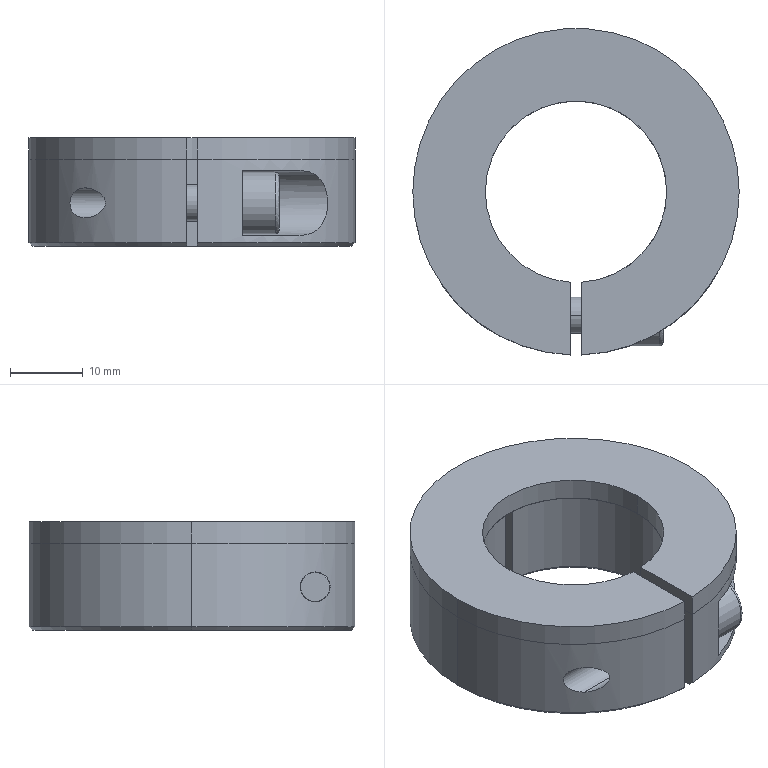Part | SolidWorks | features BaseBody 3 | 3 solids | 68 faces | box 45 x 44.987 x 15 mm | volume 15909 mm3 | plane 29 | cylinder 21 | cone 12 | spline 6 | commonest cylinder face diameters 25 x6 45 x6 4.134 x2 5 x2 5.5 x2 8.5 x2